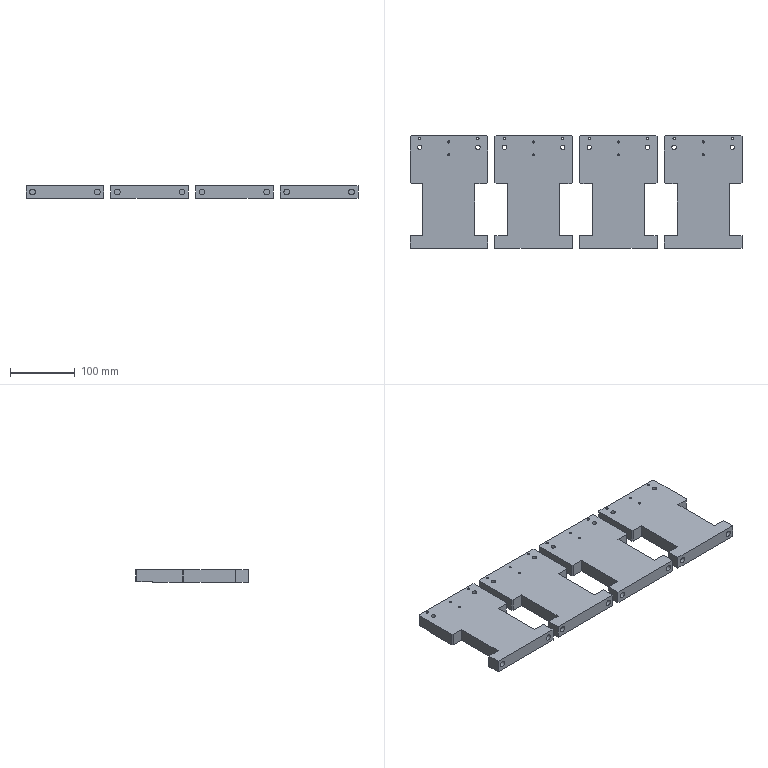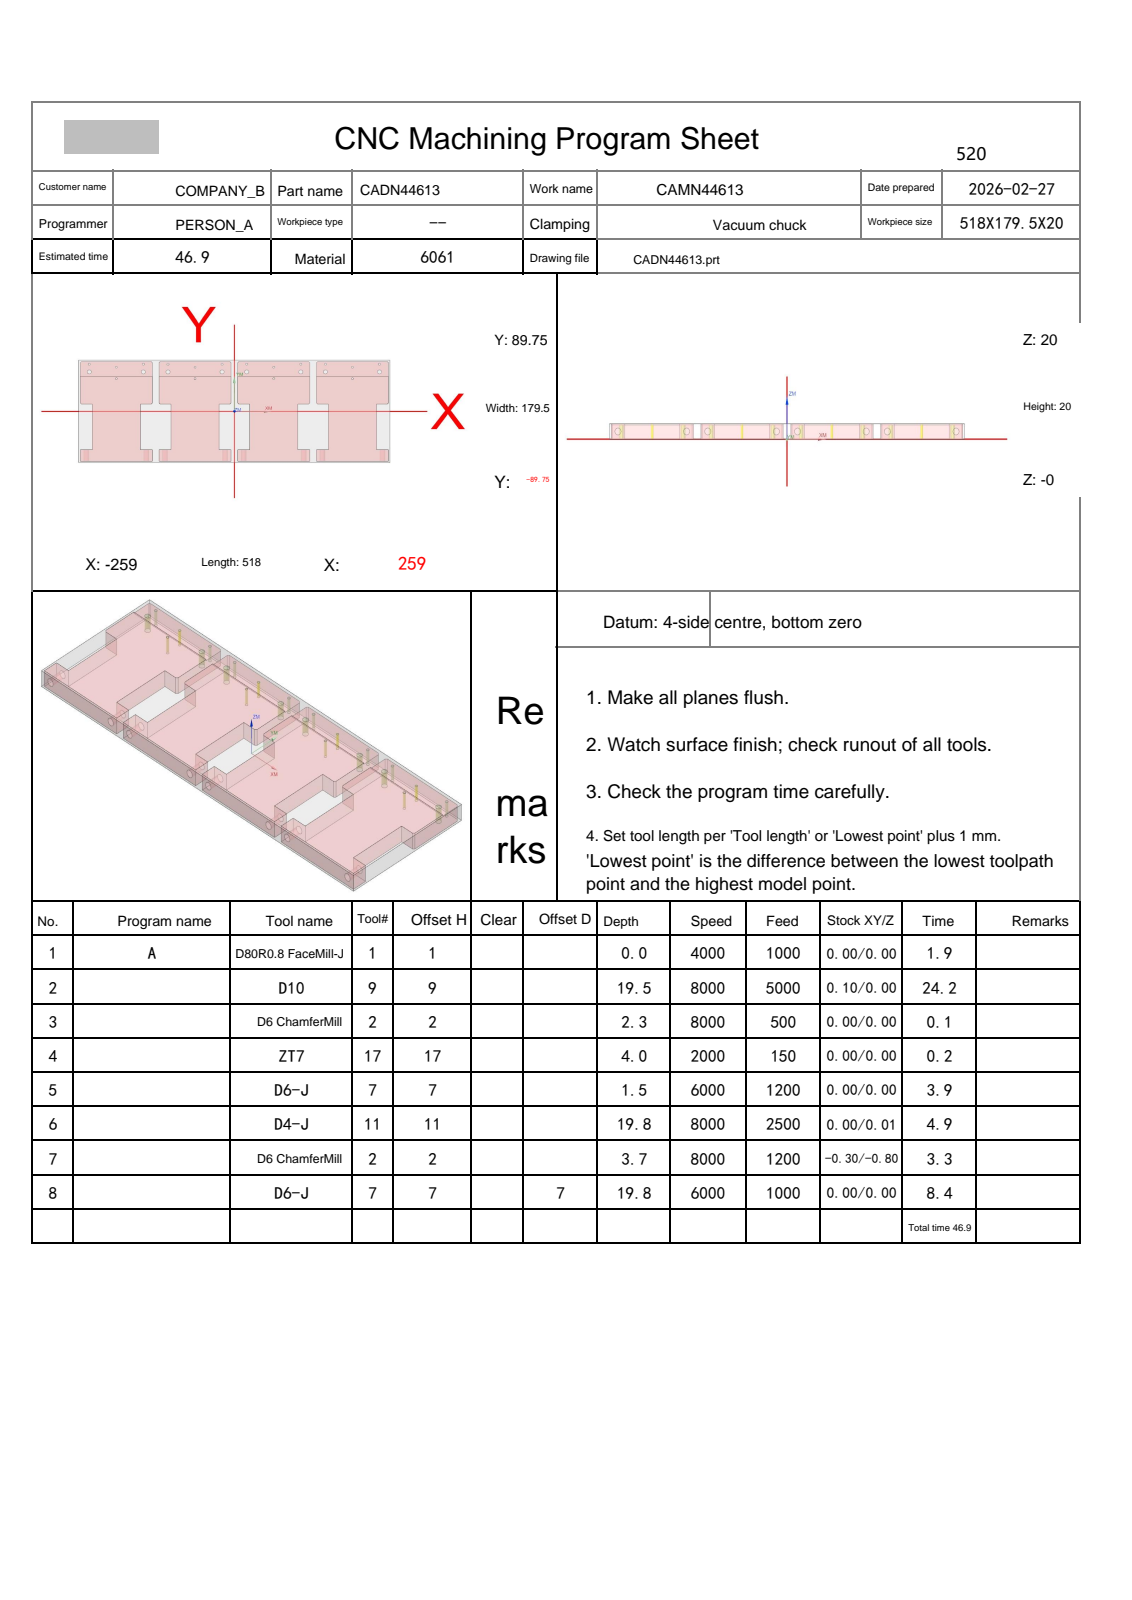NC program | NX | posted by the shop | part box 513 x 174.5 x 20 mm
Lines 1 to 40 of 36838:
%
O0001
(Machine time: 48.41 MIN)
(===Total Tool:6===)
(T1=D80R0.8 FaceMill-J D=80.  R=0.8  D-  H01 Z=20.   )
(T9=D10     D=10.  R=0.   D-  H09 Z=0.5   )
(T2=D6 ChamferMill   D=6.   R=0.   D-  H02 Z=16.3  )
(T17=ZT7    D=7.   DR_a=118 D-  H17 Z=16.   )
(T7=D6-J    D=6.   R=0.   D7  H07 Z=0.2   )
(T11=D4-J   D=4.   R=0.   D-  H11 Z=0.2   )
G80 G90 G17 G49 G40
G91 G28 Z0
M01
N1 T01 M06
(D80R0.8 FaceMill-J  D=80. R=0.8 H=01 ce=0.00 di=0.00)
G00 G90 G54 X-308.499 Y63.249 M03 S4000
G43 H01 Z50.
M08
Z22.
G01 Z20. F1000.
X-296.499
X288.504
G02 X296.499 Y55.254 I-.005 J-8.
G01 Y11.675
G02 X288.504 Y3.68 I-8. J.005
G01 X-288.504
G03 X-296.499 Y-4.315 I.005 J-8.
G01 Y-47.894
G03 X-288.504 Y-55.889 I8. J.005
G01 X296.499
X308.499
Z22.
G00 Z50.
G91 G28 Z0.0
M05
M09
G91 G28 Z0.0
M01